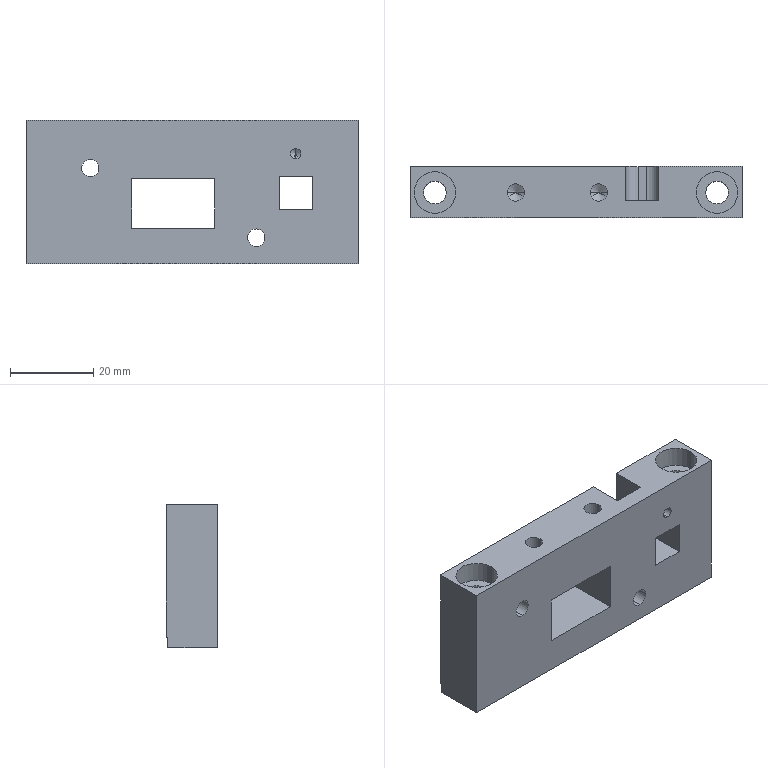Part | STEP file | detection side block left | 1 solid | 48 faces | box 80 x 12.3 x 34.5 mm | volume 25865 mm3 | plane 22 | cylinder 20 | cone 6 | commonest cylinder face diameters 4.2 x8 5.5 x4 10 x4 2.5 x2 6 x2